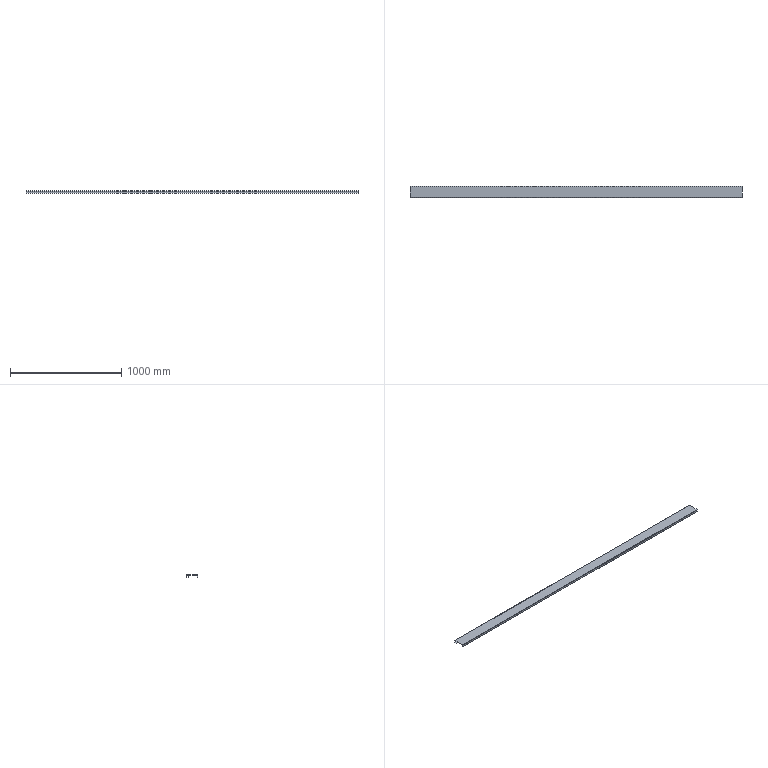Part | STEP file | E3-Transfer kettle guardrail 1 toe plate | 1 solid | 18 faces | box 2980 x 100 x 20 mm | volume 685013 mm3 | plane 12 | cylinder 6 | commonest cylinder face diameters 2 x3 5 x3
STEP:
#1=CARTESIAN_POINT('',(0.,0.,0.));
#2=DIRECTION('',(0.,0.,1.));
#3=DIRECTION('',(1.,0.,0.));
#4=AXIS2_PLACEMENT_3D('',#1,#2,#3);
#5=CARTESIAN_POINT('',(-1490.,1.5,-2.5));
#6=VERTEX_POINT('',#5);
#7=CARTESIAN_POINT('',(-1490.,1.5,-20.));
#8=VERTEX_POINT('',#7);
#9=CARTESIAN_POINT('',(-1490.,1.5,-2.5));
#10=DIRECTION('',(0.,0.,-1.));
#11=VECTOR('',#10,1.);
#12=LINE('',#9,#11);
#13=CARTESIAN_POINT('',(1490.,1.5,-2.5));
#14=DIRECTION('',(0.,-1.,0.));
#15=DIRECTION('',(0.,0.,1.));
#16=AXIS2_PLACEMENT_3D('',#13,#14,#15);
#17=PLANE('',#16);
#18=CARTESIAN_POINT('',(0.,2980.));
#19=DIRECTION('',(-1.,0.));
#20=VECTOR('',#19,1.);
#21=LINE('',#18,#20);
#22=(GEOMETRIC_REPRESENTATION_CONTEXT(2)PARAMETRIC_REPRESENTATION_CONTEXT()REPRESENTATION_CONTEXT('',''));
#23=DEFINITIONAL_REPRESENTATION('',(#21),#22);
#24=PCURVE('',#17,#23);
#25=CARTESIAN_POINT('',(-1490.,2.5,-2.5));
#26=DIRECTION('',(-1.,0.,0.));
#27=DIRECTION('',(0.,0.,-1.));
#28=AXIS2_PLACEMENT_3D('',#25,#26,#27);
#29=PLANE('',#28);
#30=CARTESIAN_POINT('',(0.,1.));
#31=DIRECTION('',(1.,0.));
#32=VECTOR('',#31,1.);
#33=LINE('',#30,#32);
#34=(GEOMETRIC_REPRESENTATION_CONTEXT(2)PARAMETRIC_REPRESENTATION_CONTEXT()REPRESENTATION_CONTEXT('',''));
#35=DEFINITIONAL_REPRESENTATION('',(#33),#34);
#36=PCURVE('',#29,#35);
#37=SURFACE_CURVE('',#12,(#24,#36),.PCURVE_S1.);
#38=EDGE_CURVE('',#6,#8,#37,.T.);
#39=ORIENTED_EDGE('',*,*,#38,.F.);
#40=CARTESIAN_POINT('',(1490.,1.5,-2.5));
#41=VERTEX_POINT('',#40);
#42=CARTESIAN_POINT('',(1490.,1.5,-2.5));
#43=DIRECTION('',(-1.,0.,0.));
#44=VECTOR('',#43,1.);
#45=LINE('',#42,#44);
#46=CARTESIAN_POINT('',(0.,0.));
#47=DIRECTION('',(0.,1.));
#48=VECTOR('',#47,1.);
#49=LINE('',#46,#48);
#50=(GEOMETRIC_REPRESENTATION_CONTEXT(2)PARAMETRIC_REPRESENTATION_CONTEXT()REPRESENTATION_CONTEXT('',''));
#51=DEFINITIONAL_REPRESENTATION('',(#49),#50);
#52=PCURVE('',#17,#51);
#53=CARTESIAN_POINT('',(1490.,2.5,-2.5));
#54=DIRECTION('',(-1.,0.,0.));
#55=DIRECTION('',(0.,0.,-1.));
#56=AXIS2_PLACEMENT_3D('',#53,#54,#55);
#57=CYLINDRICAL_SURFACE('',#56,1.);
#58=CARTESIAN_POINT('',(1.571,0.));
#59=DIRECTION('',(0.,1.));
#60=VECTOR('',#59,1.);
#61=LINE('',#58,#60);
#62=(GEOMETRIC_REPRESENTATION_CONTEXT(2)PARAMETRIC_REPRESENTATION_CONTEXT()REPRESENTATION_CONTEXT('',''));
#63=DEFINITIONAL_REPRESENTATION('',(#61),#62);
#64=PCURVE('',#57,#63);
#65=SURFACE_CURVE('',#45,(#52,#64),.PCURVE_S1.);
#66=EDGE_CURVE('',#41,#6,#65,.T.);
#67=ORIENTED_EDGE('',*,*,#66,.F.);
#68=CARTESIAN_POINT('',(1490.,1.5,-20.));
#69=VERTEX_POINT('',#68);
#70=CARTESIAN_POINT('',(1490.,1.5,-2.5));
#71=DIRECTION('',(0.,0.,-1.));
#72=VECTOR('',#71,1.);
#73=LINE('',#70,#72);
#74=CARTESIAN_POINT('',(0.,0.));
#75=DIRECTION('',(-1.,0.));
#76=VECTOR('',#75,1.);
#77=LINE('',#74,#76);
#78=(GEOMETRIC_REPRESENTATION_CONTEXT(2)PARAMETRIC_REPRESENTATION_CONTEXT()REPRESENTATION_CONTEXT('',''));
#79=DEFINITIONAL_REPRESENTATION('',(#77),#78);
#80=PCURVE('',#17,#79);
#81=CARTESIAN_POINT('',(1490.,2.5,-2.5));
#82=DIRECTION('',(-1.,0.,0.));
#83=DIRECTION('',(0.,0.,-1.));
#84=AXIS2_PLACEMENT_3D('',#81,#82,#83);
#85=PLANE('',#84);
#86=CARTESIAN_POINT('',(0.,1.));
#87=DIRECTION('',(1.,0.));
#88=VECTOR('',#87,1.);
#89=LINE('',#86,#88);
#90=(GEOMETRIC_REPRESENTATION_CONTEXT(2)PARAMETRIC_REPRESENTATION_CONTEXT()REPRESENTATION_CONTEXT('',''));
#91=DEFINITIONAL_REPRESENTATION('',(#89),#90);
#92=PCURVE('',#85,#91);
#93=SURFACE_CURVE('',#73,(#80,#92),.PCURVE_S1.);
#94=EDGE_CURVE('',#41,#69,#93,.T.);
#95=ORIENTED_EDGE('',*,*,#94,.T.);
#96=CARTESIAN_POINT('',(1490.,1.5,-20.));
#97=DIRECTION('',(-1.,0.,0.));
#98=VECTOR('',#97,1.);
#99=LINE('',#96,#98);
#100=CARTESIAN_POINT('',(-17.5,0.));
#101=DIRECTION('',(0.,1.));
#102=VECTOR('',#101,1.);
#103=LINE('',#100,#102);
#104=(GEOMETRIC_REPRESENTATION_CONTEXT(2)PARAMETRIC_REPRESENTATION_CONTEXT()REPRESENTATION_CONTEXT('',''));
#105=DEFINITIONAL_REPRESENTATION('',(#103),#104);
#106=PCURVE('',#17,#105);
#107=CARTESIAN_POINT('',(1490.,0.,-20.));
#108=DIRECTION('',(0.,0.,-1.));
#109=DIRECTION('',(1.,0.,0.));
#110=AXIS2_PLACEMENT_3D('',#107,#108,#109);
#111=PLANE('',#110);
#112=CARTESIAN_POINT('',(0.,-1.5));
#113=DIRECTION('',(-1.,0.));
#114=VECTOR('',#113,1.);
#115=LINE('',#112,#114);
#116=(GEOMETRIC_REPRESENTATION_CONTEXT(2)PARAMETRIC_REPRESENTATION_CONTEXT()REPRESENTATION_CONTEXT('',''));
#117=DEFINITIONAL_REPRESENTATION('',(#115),#116);
#118=PCURVE('',#111,#117);
#119=SURFACE_CURVE('',#99,(#106,#118),.PCURVE_S1.);
#120=EDGE_CURVE('',#69,#8,#119,.T.);
#121=ORIENTED_EDGE('',*,*,#120,.T.);
#122=EDGE_LOOP('',(#39,#67,#95,#121));
#123=FACE_BOUND('',#122,.T.);
#124=ADVANCED_FACE('',(#123),#17,.F.);
#125=CARTESIAN_POINT('',(-1490.,0.,-20.));
#126=VERTEX_POINT('',#125);
#127=CARTESIAN_POINT('',(-1490.,0.,-20.));
#128=DIRECTION('',(0.,1.,0.));
#129=VECTOR('',#128,1.);
#130=LINE('',#127,#129);
#131=CARTESIAN_POINT('',(-2980.,0.));
#132=DIRECTION('',(0.,-1.));
#133=VECTOR('',#132,1.);
#134=LINE('',#131,#133);
#135=(GEOMETRIC_REPRESENTATION_CONTEXT(2)PARAMETRIC_REPRESENTATION_CONTEXT()REPRESENTATION_CONTEXT('',''));
#136=DEFINITIONAL_REPRESENTATION('',(#134),#135);
#137=PCURVE('',#111,#136);
#138=CARTESIAN_POINT('',(17.5,2.5));
#139=DIRECTION('',(0.,-1.));
#140=VECTOR('',#139,1.);
#141=LINE('',#138,#140);
#142=(GEOMETRIC_REPRESENTATION_CONTEXT(2)PARAMETRIC_REPRESENTATION_CONTEXT()REPRESENTATION_CONTEXT('',''));
#143=DEFINITIONAL_REPRESENTATION('',(#141),#142);
#144=PCURVE('',#29,#143);
#145=SURFACE_CURVE('',#130,(#137,#144),.PCURVE_S1.);
#146=EDGE_CURVE('',#126,#8,#145,.T.);
#147=ORIENTED_EDGE('',*,*,#146,.T.);
#148=ORIENTED_EDGE('',*,*,#120,.F.);
#149=CARTESIAN_POINT('',(1490.,0.,-20.));
#150=VERTEX_POINT('',#149);
#151=CARTESIAN_POINT('',(1490.,0.,-20.));
#152=DIRECTION('',(0.,1.,0.));
#153=VECTOR('',#152,1.);
#154=LINE('',#151,#153);
#155=CARTESIAN_POINT('',(0.,0.));
#156=DIRECTION('',(0.,-1.));
#157=VECTOR('',#156,1.);
#158=LINE('',#155,#157);
#159=(GEOMETRIC_REPRESENTATION_CONTEXT(2)PARAMETRIC_REPRESENTATION_CONTEXT()REPRESENTATION_CONTEXT('',''));
#160=DEFINITIONAL_REPRESENTATION('',(#158),#159);
#161=PCURVE('',#111,#160);
#162=CARTESIAN_POINT('',(17.5,2.5));
#163=DIRECTION('',(0.,-1.));
#164=VECTOR('',#163,1.);
#165=LINE('',#162,#164);
#166=(GEOMETRIC_REPRESENTATION_CONTEXT(2)PARAMETRIC_REPRESENTATION_CONTEXT()REPRESENTATION_CONTEXT('',''));
#167=DEFINITIONAL_REPRESENTATION('',(#165),#166);
#168=PCURVE('',#85,#167);
#169=SURFACE_CURVE('',#154,(#161,#168),.PCURVE_S1.);
#170=EDGE_CURVE('',#150,#69,#169,.T.);
#171=ORIENTED_EDGE('',*,*,#170,.F.);
#172=CARTESIAN_POINT('',(1490.,0.,-20.));
#173=DIRECTION('',(-1.,0.,0.));
#174=VECTOR('',#173,1.);
#175=LINE('',#172,#174);
#176=CARTESIAN_POINT('',(0.,0.));
#177=DIRECTION('',(-1.,0.));
#178=VECTOR('',#177,1.);
#179=LINE('',#176,#178);
#180=(GEOMETRIC_REPRESENTATION_CONTEXT(2)PARAMETRIC_REPRESENTATION_CONTEXT()REPRESENTATION_CONTEXT('',''));
#181=DEFINITIONAL_REPRESENTATION('',(#179),#180);
#182=PCURVE('',#111,#181);
#183=CARTESIAN_POINT('',(1490.,0.,-2.5));
#184=DIRECTION('',(0.,-1.,0.));
#185=DIRECTION('',(0.,0.,1.));
#186=AXIS2_PLACEMENT_3D('',#183,#184,#185);
#187=PLANE('',#186);
#188=CARTESIAN_POINT('',(-17.5,0.));
#189=DIRECTION('',(0.,1.));
#190=VECTOR('',#189,1.);
#191=LINE('',#188,#190);
#192=(GEOMETRIC_REPRESENTATION_CONTEXT(2)PARAMETRIC_REPRESENTATION_CONTEXT()REPRESENTATION_CONTEXT('',''));
#193=DEFINITIONAL_REPRESENTATION('',(#191),#192);
#194=PCURVE('',#187,#193);
#195=SURFACE_CURVE('',#175,(#182,#194),.PCURVE_S1.);
#196=EDGE_CURVE('',#150,#126,#195,.T.);
#197=ORIENTED_EDGE('',*,*,#196,.T.);
#198=EDGE_LOOP('',(#147,#148,#171,#197));
#199=FACE_BOUND('',#198,.T.);
#200=ADVANCED_FACE('',(#199),#111,.T.);
#201=CARTESIAN_POINT('',(-1490.,0.,-2.5));
#202=VERTEX_POINT('',#201);
#203=CARTESIAN_POINT('',(-1490.,0.,-2.5));
#204=DIRECTION('',(0.,0.,-1.));
#205=VECTOR('',#204,1.);
#206=LINE('',#203,#205);
#207=CARTESIAN_POINT('',(0.,2980.));
#208=DIRECTION('',(-1.,0.));
#209=VECTOR('',#208,1.);
#210=LINE('',#207,#209);
#211=(GEOMETRIC_REPRESENTATION_CONTEXT(2)PARAMETRIC_REPRESENTATION_CONTEXT()REPRESENTATION_CONTEXT('',''));
#212=DEFINITIONAL_REPRESENTATION('',(#210),#211);
#213=PCURVE('',#187,#212);
#214=CARTESIAN_POINT('',(0.,2.5));
#215=DIRECTION('',(1.,0.));
#216=VECTOR('',#215,1.);
#217=LINE('',#214,#216);
#218=(GEOMETRIC_REPRESENTATION_CONTEXT(2)PARAMETRIC_REPRESENTATION_CONTEXT()REPRESENTATION_CONTEXT('',''));
#219=DEFINITIONAL_REPRESENTATION('',(#217),#218);
#220=PCURVE('',#29,#219);
#221=SURFACE_CURVE('',#206,(#213,#220),.PCURVE_S1.);
#222=EDGE_CURVE('',#202,#126,#221,.T.);
#223=ORIENTED_EDGE('',*,*,#222,.T.);
#224=ORIENTED_EDGE('',*,*,#196,.F.);
#225=CARTESIAN_POINT('',(1490.,0.,-2.5));
#226=VERTEX_POINT('',#225);
#227=CARTESIAN_POINT('',(1490.,0.,-2.5));
#228=DIRECTION('',(0.,0.,-1.));
#229=VECTOR('',#228,1.);
#230=LINE('',#227,#229);
#231=CARTESIAN_POINT('',(0.,0.));
#232=DIRECTION('',(-1.,0.));
#233=VECTOR('',#232,1.);
#234=LINE('',#231,#233);
#235=(GEOMETRIC_REPRESENTATION_CONTEXT(2)PARAMETRIC_REPRESENTATION_CONTEXT()REPRESENTATION_CONTEXT('',''));
#236=DEFINITIONAL_REPRESENTATION('',(#234),#235);
#237=PCURVE('',#187,#236);
#238=CARTESIAN_POINT('',(0.,2.5));
#239=DIRECTION('',(1.,0.));
#240=VECTOR('',#239,1.);
#241=LINE('',#238,#240);
#242=(GEOMETRIC_REPRESENTATION_CONTEXT(2)PARAMETRIC_REPRESENTATION_CONTEXT()REPRESENTATION_CONTEXT('',''));
#243=DEFINITIONAL_REPRESENTATION('',(#241),#242);
#244=PCURVE('',#85,#243);
#245=SURFACE_CURVE('',#230,(#237,#244),.PCURVE_S1.);
#246=EDGE_CURVE('',#226,#150,#245,.T.);
#247=ORIENTED_EDGE('',*,*,#246,.F.);
#248=CARTESIAN_POINT('',(1490.,0.,-2.5));
#249=DIRECTION('',(-1.,0.,0.));
#250=VECTOR('',#249,1.);
#251=LINE('',#248,#250);
#252=CARTESIAN_POINT('',(0.,0.));
#253=DIRECTION('',(0.,1.));
#254=VECTOR('',#253,1.);
#255=LINE('',#252,#254);
#256=(GEOMETRIC_REPRESENTATION_CONTEXT(2)PARAMETRIC_REPRESENTATION_CONTEXT()REPRESENTATION_CONTEXT('',''));
#257=DEFINITIONAL_REPRESENTATION('',(#255),#256);
#258=PCURVE('',#187,#257);
#259=CARTESIAN_POINT('',(1490.,2.5,-2.5));
#260=DIRECTION('',(-1.,0.,0.));
#261=DIRECTION('',(0.,0.,-1.));
#262=AXIS2_PLACEMENT_3D('',#259,#260,#261);
#263=CYLINDRICAL_SURFACE('',#262,2.5);
#264=CARTESIAN_POINT('',(1.571,0.));
#265=DIRECTION('',(0.,1.));
#266=VECTOR('',#265,1.);
#267=LINE('',#264,#266);
#268=(GEOMETRIC_REPRESENTATION_CONTEXT(2)PARAMETRIC_REPRESENTATION_CONTEXT()REPRESENTATION_CONTEXT('',''));
#269=DEFINITIONAL_REPRESENTATION('',(#267),#268);
#270=PCURVE('',#263,#269);
#271=SURFACE_CURVE('',#251,(#258,#270),.PCURVE_S1.);
#272=EDGE_CURVE('',#226,#202,#271,.T.);
#273=ORIENTED_EDGE('',*,*,#272,.T.);
#274=EDGE_LOOP('',(#223,#224,#247,#273));
#275=FACE_BOUND('',#274,.T.);
#276=ADVANCED_FACE('',(#275),#187,.T.);
#277=CARTESIAN_POINT('',(-1490.,2.5,0.));
#278=VERTEX_POINT('',#277);
#279=CARTESIAN_POINT('',(-1490.,2.5,-2.5));
#280=DIRECTION('',(1.,0.,0.));
#281=DIRECTION('',(0.,0.,-1.));
#282=AXIS2_PLACEMENT_3D('',#279,#280,#281);
#283=CIRCLE('',#282,2.5);
#284=CARTESIAN_POINT('',(6.283,2980.));
#285=DIRECTION('',(-1.,0.));
#286=VECTOR('',#285,1.);
#287=LINE('',#284,#286);
#288=(GEOMETRIC_REPRESENTATION_CONTEXT(2)PARAMETRIC_REPRESENTATION_CONTEXT()REPRESENTATION_CONTEXT('',''));
#289=DEFINITIONAL_REPRESENTATION('',(#287),#288);
#290=PCURVE('',#263,#289);
#291=CARTESIAN_POINT('',(2.5,0.));
#292=CARTESIAN_POINT('',(2.5,-4.33));
#293=CARTESIAN_POINT('',(-1.25,-2.165));
#294=CARTESIAN_POINT('',(-5.,0.));
#295=CARTESIAN_POINT('',(-1.25,2.165));
#296=CARTESIAN_POINT('',(2.5,4.33));
#297=CARTESIAN_POINT('',(2.5,0.));
#298=(BOUNDED_CURVE()B_SPLINE_CURVE(2,(#291,#292,#293,#294,#295,#296,#297),.UNSPECIFIED.,.T.,.F.)B_SPLINE_CURVE_WITH_KNOTS((1,2,2,2,2,1),(-2.094,0.,2.094,4.189,6.283,8.378),.UNSPECIFIED.)CURVE()GEOMETRIC_REPRESENTATION_ITEM()RATIONAL_B_SPLINE_CURVE((1.,0.5,1.,0.5,1.,0.5,1.))REPRESENTATION_ITEM(''));
#299=(GEOMETRIC_REPRESENTATION_CONTEXT(2)PARAMETRIC_REPRESENTATION_CONTEXT()REPRESENTATION_CONTEXT('',''));
#300=DEFINITIONAL_REPRESENTATION('',(#298),#299);
#301=PCURVE('',#29,#300);
#302=SURFACE_CURVE('',#283,(#290,#301),.PCURVE_S1.);
#303=EDGE_CURVE('',#278,#202,#302,.T.);
#304=ORIENTED_EDGE('',*,*,#303,.T.);
#305=ORIENTED_EDGE('',*,*,#272,.F.);
#306=CARTESIAN_POINT('',(1490.,2.5,0.));
#307=VERTEX_POINT('',#306);
#308=CARTESIAN_POINT('',(1490.,2.5,-2.5));
#309=DIRECTION('',(1.,0.,0.));
#310=DIRECTION('',(0.,0.,-1.));
#311=AXIS2_PLACEMENT_3D('',#308,#309,#310);
#312=CIRCLE('',#311,2.5);
#313=CARTESIAN_POINT('',(6.283,0.));
#314=DIRECTION('',(-1.,0.));
#315=VECTOR('',#314,1.);
#316=LINE('',#313,#315);
#317=(GEOMETRIC_REPRESENTATION_CONTEXT(2)PARAMETRIC_REPRESENTATION_CONTEXT()REPRESENTATION_CONTEXT('',''));
#318=DEFINITIONAL_REPRESENTATION('',(#316),#317);
#319=PCURVE('',#263,#318);
#320=CARTESIAN_POINT('',(2.5,0.));
#321=CARTESIAN_POINT('',(2.5,-4.33));
#322=CARTESIAN_POINT('',(-1.25,-2.165));
#323=CARTESIAN_POINT('',(-5.,0.));
#324=CARTESIAN_POINT('',(-1.25,2.165));
#325=CARTESIAN_POINT('',(2.5,4.33));
#326=CARTESIAN_POINT('',(2.5,0.));
#327=(BOUNDED_CURVE()B_SPLINE_CURVE(2,(#320,#321,#322,#323,#324,#325,#326),.UNSPECIFIED.,.T.,.F.)B_SPLINE_CURVE_WITH_KNOTS((1,2,2,2,2,1),(-2.094,0.,2.094,4.189,6.283,8.378),.UNSPECIFIED.)CURVE()GEOMETRIC_REPRESENTATION_ITEM()RATIONAL_B_SPLINE_CURVE((1.,0.5,1.,0.5,1.,0.5,1.))REPRESENTATION_ITEM(''));
#328=(GEOMETRIC_REPRESENTATION_CONTEXT(2)PARAMETRIC_REPRESENTATION_CONTEXT()REPRESENTATION_CONTEXT('',''));
#329=DEFINITIONAL_REPRESENTATION('',(#327),#328);
#330=PCURVE('',#85,#329);
#331=SURFACE_CURVE('',#312,(#319,#330),.PCURVE_S1.);
#332=EDGE_CURVE('',#307,#226,#331,.T.);
#333=ORIENTED_EDGE('',*,*,#332,.F.);
#334=CARTESIAN_POINT('',(1490.,2.5,0.));
#335=DIRECTION('',(-1.,0.,0.));
#336=VECTOR('',#335,1.);
#337=LINE('',#334,#336);
#338=CARTESIAN_POINT('',(3.142,0.));
#339=DIRECTION('',(0.,1.));
#340=VECTOR('',#339,1.);
#341=LINE('',#338,#340);
#342=(GEOMETRIC_REPRESENTATION_CONTEXT(2)PARAMETRIC_REPRESENTATION_CONTEXT()REPRESENTATION_CONTEXT('',''));
#343=DEFINITIONAL_REPRESENTATION('',(#341),#342);
#344=PCURVE('',#263,#343);
#345=CARTESIAN_POINT('',(1490.,2.5,0.));
#346=DIRECTION('',(0.,0.,1.));
#347=DIRECTION('',(-1.,0.,0.));
#348=AXIS2_PLACEMENT_3D('',#345,#346,#347);
#349=PLANE('',#348);
#350=CARTESIAN_POINT('',(0.,0.));
#351=DIRECTION('',(1.,0.));
#352=VECTOR('',#351,1.);
#353=LINE('',#350,#352);
#354=(GEOMETRIC_REPRESENTATION_CONTEXT(2)PARAMETRIC_REPRESENTATION_CONTEXT()REPRESENTATION_CONTEXT('',''));
#355=DEFINITIONAL_REPRESENTATION('',(#353),#354);
#356=PCURVE('',#349,#355);
#357=SURFACE_CURVE('',#337,(#344,#356),.PCURVE_S1.);
#358=EDGE_CURVE('',#307,#278,#357,.T.);
#359=ORIENTED_EDGE('',*,*,#358,.T.);
#360=EDGE_LOOP('',(#304,#305,#333,#359));
#361=FACE_BOUND('',#360,.T.);
#362=ADVANCED_FACE('',(#361),#263,.T.);
#363=CARTESIAN_POINT('',(-1490.,97.5,0.));
#364=VERTEX_POINT('',#363);
#365=CARTESIAN_POINT('',(-1490.,2.5,0.));
#366=DIRECTION('',(0.,-1.,0.));
#367=VECTOR('',#366,1.);
#368=LINE('',#365,#367);
#369=CARTESIAN_POINT('',(2980.,0.));
#370=DIRECTION('',(0.,1.));
#371=VECTOR('',#370,1.);
#372=LINE('',#369,#371);
#373=(GEOMETRIC_REPRESENTATION_CONTEXT(2)PARAMETRIC_REPRESENTATION_CONTEXT()REPRESENTATION_CONTEXT('',''));
#374=DEFINITIONAL_REPRESENTATION('',(#372),#373);
#375=PCURVE('',#349,#374);
#376=CARTESIAN_POINT('',(-2.5,0.));
#377=DIRECTION('',(0.,1.));
#378=VECTOR('',#377,1.);
#379=LINE('',#376,#378);
#380=(GEOMETRIC_REPRESENTATION_CONTEXT(2)PARAMETRIC_REPRESENTATION_CONTEXT()REPRESENTATION_CONTEXT('',''));
#381=DEFINITIONAL_REPRESENTATION('',(#379),#380);
#382=PCURVE('',#29,#381);
#383=SURFACE_CURVE('',#368,(#375,#382),.PCURVE_S1.);
#384=EDGE_CURVE('',#364,#278,#383,.T.);
#385=ORIENTED_EDGE('',*,*,#384,.T.);
#386=ORIENTED_EDGE('',*,*,#358,.F.);
#387=CARTESIAN_POINT('',(1490.,97.5,0.));
#388=VERTEX_POINT('',#387);
#389=CARTESIAN_POINT('',(1490.,2.5,0.));
#390=DIRECTION('',(0.,-1.,0.));
#391=VECTOR('',#390,1.);
#392=LINE('',#389,#391);
#393=CARTESIAN_POINT('',(0.,0.));
#394=DIRECTION('',(0.,1.));
#395=VECTOR('',#394,1.);
#396=LINE('',#393,#395);
#397=(GEOMETRIC_REPRESENTATION_CONTEXT(2)PARAMETRIC_REPRESENTATION_CONTEXT()REPRESENTATION_CONTEXT('',''));
#398=DEFINITIONAL_REPRESENTATION('',(#396),#397);
#399=PCURVE('',#349,#398);
#400=CARTESIAN_POINT('',(-2.5,0.));
#401=DIRECTION('',(0.,1.));
#402=VECTOR('',#401,1.);
#403=LINE('',#400,#402);
#404=(GEOMETRIC_REPRESENTATION_CONTEXT(2)PARAMETRIC_REPRESENTATION_CONTEXT()REPRESENTATION_CONTEXT('',''));
#405=DEFINITIONAL_REPRESENTATION('',(#403),#404);
#406=PCURVE('',#85,#405);
#407=SURFACE_CURVE('',#392,(#399,#406),.PCURVE_S1.);
#408=EDGE_CURVE('',#388,#307,#407,.T.);
#409=ORIENTED_EDGE('',*,*,#408,.F.);
#410=CARTESIAN_POINT('',(1490.,97.5,0.));
#411=DIRECTION('',(-1.,0.,0.));
#412=VECTOR('',#411,1.);
#413=LINE('',#410,#412);
#414=CARTESIAN_POINT('',(0.,-95.));
#415=DIRECTION('',(1.,0.));
#416=VECTOR('',#415,1.);
#417=LINE('',#414,#416);
#418=(GEOMETRIC_REPRESENTATION_CONTEXT(2)PARAMETRIC_REPRESENTATION_CONTEXT()REPRESENTATION_CONTEXT('',''));
#419=DEFINITIONAL_REPRESENTATION('',(#417),#418);
#420=PCURVE('',#349,#419);
#421=CARTESIAN_POINT('',(1490.,97.5,-2.5));
#422=DIRECTION('',(-1.,0.,0.));
#423=DIRECTION('',(0.,0.,-1.));
#424=AXIS2_PLACEMENT_3D('',#421,#422,#423);
#425=CYLINDRICAL_SURFACE('',#424,2.5);
#426=CARTESIAN_POINT('',(3.142,0.));
#427=DIRECTION('',(0.,1.));
#428=VECTOR('',#427,1.);
#429=LINE('',#426,#428);
#430=(GEOMETRIC_REPRESENTATION_CONTEXT(2)PARAMETRIC_REPRESENTATION_CONTEXT()REPRESENTATION_CONTEXT('',''));
#431=DEFINITIONAL_REPRESENTATION('',(#429),#430);
#432=PCURVE('',#425,#431);
#433=SURFACE_CURVE('',#413,(#420,#432),.PCURVE_S1.);
#434=EDGE_CURVE('',#388,#364,#433,.T.);
#435=ORIENTED_EDGE('',*,*,#434,.T.);
#436=EDGE_LOOP('',(#385,#386,#409,#435));
#437=FACE_BOUND('',#436,.T.);
#438=ADVANCED_FACE('',(#437),#349,.T.);
#439=CARTESIAN_POINT('',(-1490.,100.,-2.5));
#440=VERTEX_POINT('',#439);
#441=CARTESIAN_POINT('',(-1490.,97.5,-2.5));
#442=DIRECTION('',(1.,0.,0.));
#443=DIRECTION('',(0.,0.,1.));
#444=AXIS2_PLACEMENT_3D('',#441,#442,#443);
#445=CIRCLE('',#444,2.5);
#446=CARTESIAN_POINT('',(9.425,2980.));
#447=DIRECTION('',(-1.,0.));
#448=VECTOR('',#447,1.);
#449=LINE('',#446,#448);
#450=(GEOMETRIC_REPRESENTATION_CONTEXT(2)PARAMETRIC_REPRESENTATION_CONTEXT()REPRESENTATION_CONTEXT('',''));
#451=DEFINITIONAL_REPRESENTATION('',(#449),#450);
#452=PCURVE('',#425,#451);
#453=CARTESIAN_POINT('',(-2.5,-95.));
#454=CARTESIAN_POINT('',(-2.5,-90.67));
#455=CARTESIAN_POINT('',(1.25,-92.835));
#456=CARTESIAN_POINT('',(5.,-95.));
#457=CARTESIAN_POINT('',(1.25,-97.165));
#458=CARTESIAN_POINT('',(-2.5,-99.33));
#459=CARTESIAN_POINT('',(-2.5,-95.));
#460=(BOUNDED_CURVE()B_SPLINE_CURVE(2,(#453,#454,#455,#456,#457,#458,#459),.UNSPECIFIED.,.T.,.F.)B_SPLINE_CURVE_WITH_KNOTS((1,2,2,2,2,1),(-2.094,0.,2.094,4.189,6.283,8.378),.UNSPECIFIED.)CURVE()GEOMETRIC_REPRESENTATION_ITEM()RATIONAL_B_SPLINE_CURVE((1.,0.5,1.,0.5,1.,0.5,1.))REPRESENTATION_ITEM(''));
#461=(GEOMETRIC_REPRESENTATION_CONTEXT(2)PARAMETRIC_REPRESENTATION_CONTEXT()REPRESENTATION_CONTEXT('',''));
#462=DEFINITIONAL_REPRESENTATION('',(#460),#461);
#463=PCURVE('',#29,#462);
#464=SURFACE_CURVE('',#445,(#452,#463),.PCURVE_S1.);
#465=EDGE_CURVE('',#440,#364,#464,.T.);
#466=ORIENTED_EDGE('',*,*,#465,.T.);
#467=ORIENTED_EDGE('',*,*,#434,.F.);
#468=CARTESIAN_POINT('',(1490.,100.,-2.5));
#469=VERTEX_POINT('',#468);
#470=CARTESIAN_POINT('',(1490.,97.5,-2.5));
#471=DIRECTION('',(1.,0.,0.));
#472=DIRECTION('',(0.,0.,1.));
#473=AXIS2_PLACEMENT_3D('',#470,#471,#472);
#474=CIRCLE('',#473,2.5);
#475=CARTESIAN_POINT('',(9.425,0.));
#476=DIRECTION('',(-1.,0.));
#477=VECTOR('',#476,1.);
#478=LINE('',#475,#477);
#479=(GEOMETRIC_REPRESENTATION_CONTEXT(2)PARAMETRIC_REPRESENTATION_CONTEXT()REPRESENTATION_CONTEXT('',''));
#480=DEFINITIONAL_REPRESENTATION('',(#478),#479);
#481=PCURVE('',#425,#480);
#482=CARTESIAN_POINT('',(-2.5,-95.));
#483=CARTESIAN_POINT('',(-2.5,-90.67));
#484=CARTESIAN_POINT('',(1.25,-92.835));
#485=CARTESIAN_POINT('',(5.,-95.));
#486=CARTESIAN_POINT('',(1.25,-97.165));
#487=CARTESIAN_POINT('',(-2.5,-99.33));
#488=CARTESIAN_POINT('',(-2.5,-95.));
#489=(BOUNDED_CURVE()B_SPLINE_CURVE(2,(#482,#483,#484,#485,#486,#487,#488),.UNSPECIFIED.,.T.,.F.)B_SPLINE_CURVE_WITH_KNOTS((1,2,2,2,2,1),(-2.094,0.,2.094,4.189,6.283,8.378),.UNSPECIFIED.)CURVE()GEOMETRIC_REPRESENTATION_ITEM()RATIONAL_B_SPLINE_CURVE((1.,0.5,1.,0.5,1.,0.5,1.))REPRESENTATION_ITEM(''));
#490=(GEOMETRIC_REPRESENTATION_CONTEXT(2)PARAMETRIC_REPRESENTATION_CONTEXT()REPRESENTATION_CONTEXT('',''));
#491=DEFINITIONAL_REPRESENTATION('',(#489),#490);
#492=PCURVE('',#85,#491);
#493=SURFACE_CURVE('',#474,(#481,#492),.PCURVE_S1.);
#494=EDGE_CURVE('',#469,#388,#493,.T.);
#495=ORIENTED_EDGE('',*,*,#494,.F.);
#496=CARTESIAN_POINT('',(1490.,100.,-2.5));
#497=DIRECTION('',(-1.,0.,0.));
#498=VECTOR('',#497,1.);
#499=LINE('',#496,#498);
#500=CARTESIAN_POINT('',(4.712,0.));
#501=DIRECTION('',(0.,1.));
#502=VECTOR('',#501,1.);
#503=LINE('',#500,#502);
#504=(GEOMETRIC_REPRESENTATION_CONTEXT(2)PARAMETRIC_REPRESENTATION_CONTEXT()REPRESENTATION_CONTEXT('',''));
#505=DEFINITIONAL_REPRESENTATION('',(#503),#504);
#506=PCURVE('',#425,#505);
#507=CARTESIAN_POINT('',(1490.,100.,-2.5));
#508=DIRECTION('',(0.,1.,0.));
#509=DIRECTION('',(0.,0.,-1.));
#510=AXIS2_PLACEMENT_3D('',#507,#508,#509);
#511=PLANE('',#510);
#512=CARTESIAN_POINT('',(0.,0.));
#513=DIRECTION('',(0.,1.));
#514=VECTOR('',#513,1.);
#515=LINE('',#512,#514);
#516=(GEOMETRIC_REPRESENTATION_CONTEXT(2)PARAMETRIC_REPRESENTATION_CONTEXT()REPRESENTATION_CONTEXT('',''));
#517=DEFINITIONAL_REPRESENTATION('',(#515),#516);
#518=PCURVE('',#511,#517);
#519=SURFACE_CURVE('',#499,(#506,#518),.PCURVE_S1.);
#520=EDGE_CURVE('',#469,#440,#519,.T.);
#521=ORIENTED_EDGE('',*,*,#520,.T.);
#522=EDGE_LOOP('',(#466,#467,#495,#521));
#523=FACE_BOUND('',#522,.T.);
#524=ADVANCED_FACE('',(#523),#425,.T.);
#525=CARTESIAN_POINT('',(-1490.,100.,-17.5));
#526=VERTEX_POINT('',#525);
#527=CARTESIAN_POINT('',(-1490.,100.,-2.5));
#528=DIRECTION('',(0.,0.,1.));
#529=VECTOR('',#528,1.);
#530=LINE('',#527,#529);
#531=CARTESIAN_POINT('',(0.,2980.));
#532=DIRECTION('',(-1.,0.));
#533=VECTOR('',#532,1.);
#534=LINE('',#531,#533);
#535=(GEOMETRIC_REPRESENTATION_CONTEXT(2)PARAMETRIC_REPRESENTATION_CONTEXT()REPRESENTATION_CONTEXT('',''));
#536=DEFINITIONAL_REPRESENTATION('',(#534),#535);
#537=PCURVE('',#511,#536);
#538=CARTESIAN_POINT('',(0.,-97.5));
#539=DIRECTION('',(-1.,0.));
#540=VECTOR('',#539,1.);
#541=LINE('',#538,#540);
#542=(GEOMETRIC_REPRESENTATION_CONTEXT(2)PARAMETRIC_REPRESENTATION_CONTEXT()REPRESENTATION_CONTEXT('',''));
#543=DEFINITIONAL_REPRESENTATION('',(#541),#542);
#544=PCURVE('',#29,#543);
#545=SURFACE_CURVE('',#530,(#537,#544),.PCURVE_S1.);
#546=EDGE_CURVE('',#526,#440,#545,.T.);
#547=ORIENTED_EDGE('',*,*,#546,.T.);
#548=ORIENTED_EDGE('',*,*,#520,.F.);
#549=CARTESIAN_POINT('',(1490.,100.,-17.5));
#550=VERTEX_POINT('',#549);
#551=CARTESIAN_POINT('',(1490.,100.,-2.5));
#552=DIRECTION('',(0.,0.,1.));
#553=VECTOR('',#552,1.);
#554=LINE('',#551,#553);
#555=CARTESIAN_POINT('',(0.,0.));
#556=DIRECTION('',(-1.,0.));
#557=VECTOR('',#556,1.);
#558=LINE('',#555,#557);
#559=(GEOMETRIC_REPRESENTATION_CONTEXT(2)PARAMETRIC_REPRESENTATION_CONTEXT()REPRESENTATION_CONTEXT('',''));
#560=DEFINITIONAL_REPRESENTATION('',(#558),#559);
#561=PCURVE('',#511,#560);
#562=CARTESIAN_POINT('',(0.,-97.5));
#563=DIRECTION('',(-1.,0.));
#564=VECTOR('',#563,1.);
#565=LINE('',#562,#564);
#566=(GEOMETRIC_REPRESENTATION_CONTEXT(2)PARAMETRIC_REPRESENTATION_CONTEXT()REPRESENTATION_CONTEXT('',''));
#567=DEFINITIONAL_REPRESENTATION('',(#565),#566);
#568=PCURVE('',#85,#567);
#569=SURFACE_CURVE('',#554,(#561,#568),.PCURVE_S1.);
#570=EDGE_CURVE('',#550,#469,#569,.T.);
#571=ORIENTED_EDGE('',*,*,#570,.F.);
#572=CARTESIAN_POINT('',(1490.,100.,-17.5));
#573=DIRECTION('',(-1.,0.,0.));
#574=VECTOR('',#573,1.);
#575=LINE('',#572,#574);
#576=CARTESIAN_POINT('',(15.,0.));
#577=DIRECTION('',(0.,1.));
#578=VECTOR('',#577,1.);
#579=LINE('',#576,#578);
#580=(GEOMETRIC_REPRESENTATION_CONTEXT(2)PARAMETRIC_REPRESENTATION_CONTEXT()REPRESENTATION_CONTEXT('',''));
#581=DEFINITIONAL_REPRESENTATION('',(#579),#580);
#582=PCURVE('',#511,#581);
#583=CARTESIAN_POINT('',(1490.,97.5,-17.5));
#584=DIRECTION('',(-1.,0.,0.));
#585=DIRECTION('',(0.,0.,-1.));
#586=AXIS2_PLACEMENT_3D('',#583,#584,#585);
#587=CYLINDRICAL_SURFACE('',#586,2.5);
#588=CARTESIAN_POINT('',(4.712,0.));
#589=DIRECTION('',(0.,1.));
#590=VECTOR('',#589,1.);
#591=LINE('',#588,#590);
#592=(GEOMETRIC_REPRESENTATION_CONTEXT(2)PARAMETRIC_REPRESENTATION_CONTEXT()REPRESENTATION_CONTEXT('',''));
#593=DEFINITIONAL_REPRESENTATION('',(#591),#592);
#594=PCURVE('',#587,#593);
#595=SURFACE_CURVE('',#575,(#582,#594),.PCURVE_S1.);
#596=EDGE_CURVE('',#550,#526,#595,.T.);
#597=ORIENTED_EDGE('',*,*,#596,.T.);
#598=EDGE_LOOP('',(#547,#548,#571,#597));
#599=FACE_BOUND('',#598,.T.);
#600=ADVANCED_FACE('',(#599),#511,.T.);
#601=CARTESIAN_POINT('',(-1490.,97.5,-20.));
#602=VERTEX_POINT('',#601);
#603=CARTESIAN_POINT('',(-1490.,97.5,-17.5));
#604=DIRECTION('',(1.,0.,0.));
#605=DIRECTION('',(0.,0.,1.));
#606=AXIS2_PLACEMENT_3D('',#603,#604,#605);
#607=CIRCLE('',#606,2.5);
#608=CARTESIAN_POINT('',(9.425,2980.));
#609=DIRECTION('',(-1.,0.));
#610=VECTOR('',#609,1.);
#611=LINE('',#608,#610);
#612=(GEOMETRIC_REPRESENTATION_CONTEXT(2)PARAMETRIC_REPRESENTATION_CONTEXT()REPRESENTATION_CONTEXT('',''));
#613=DEFINITIONAL_REPRESENTATION('',(#611),#612);
#614=PCURVE('',#587,#613);
#615=CARTESIAN_POINT('',(12.5,-95.));
#616=CARTESIAN_POINT('',(12.5,-90.67));
#617=CARTESIAN_POINT('',(16.25,-92.835));
#618=CARTESIAN_POINT('',(20.,-95.));
#619=CARTESIAN_POINT('',(16.25,-97.165));
#620=CARTESIAN_POINT('',(12.5,-99.33));
#621=CARTESIAN_POINT('',(12.5,-95.));
#622=(BOUNDED_CURVE()B_SPLINE_CURVE(2,(#615,#616,#617,#618,#619,#620,#621),.UNSPECIFIED.,.T.,.F.)B_SPLINE_CURVE_WITH_KNOTS((1,2,2,2,2,1),(-2.094,0.,2.094,4.189,6.283,8.378),.UNSPECIFIED.)CURVE()GEOMETRIC_REPRESENTATION_ITEM()RATIONAL_B_SPLINE_CURVE((1.,0.5,1.,0.5,1.,0.5,1.))REPRESENTATION_ITEM(''));
#623=(GEOMETRIC_REPRESENTATION_CONTEXT(2)PARAMETRIC_REPRESENTATION_CONTEXT()REPRESENTATION_CONTEXT('',''));
#624=DEFINITIONAL_REPRESENTATION('',(#622),#623);
#625=PCURVE('',#29,#624);
#626=SURFACE_CURVE('',#607,(#614,#625),.PCURVE_S1.);
#627=EDGE_CURVE('',#602,#526,#626,.T.);
#628=ORIENTED_EDGE('',*,*,#627,.T.);
#629=ORIENTED_EDGE('',*,*,#596,.F.);
#630=CARTESIAN_POINT('',(1490.,97.5,-20.));
#631=VERTEX_POINT('',#630);
#632=CARTESIAN_POINT('',(1490.,97.5,-17.5));
#633=DIRECTION('',(1.,0.,0.));
#634=DIRECTION('',(0.,0.,1.));
#635=AXIS2_PLACEMENT_3D('',#632,#633,#634);
#636=CIRCLE('',#635,2.5);
#637=CARTESIAN_POINT('',(9.425,0.));
#638=DIRECTION('',(-1.,0.));
#639=VECTOR('',#638,1.);
#640=LINE('',#637,#639);
#641=(GEOMETRIC_REPRESENTATION_CONTEXT(2)PARAMETRIC_REPRESENTATION_CONTEXT()REPRESENTATION_CONTEXT('',''));
#642=DEFINITIONAL_REPRESENTATION('',(#640),#641);
#643=PCURVE('',#587,#642);
#644=CARTESIAN_POINT('',(12.5,-95.));
#645=CARTESIAN_POINT('',(12.5,-90.67));
#646=CARTESIAN_POINT('',(16.25,-92.835));
#647=CARTESIAN_POINT('',(20.,-95.));
#648=CARTESIAN_POINT('',(16.25,-97.165));
#649=CARTESIAN_POINT('',(12.5,-99.33));
#650=CARTESIAN_POINT('',(12.5,-95.));
#651=(BOUNDED_CURVE()B_SPLINE_CURVE(2,(#644,#645,#646,#647,#648,#649,#650),.UNSPECIFIED.,.T.,.F.)B_SPLINE_CURVE_WITH_KNOTS((1,2,2,2,2,1),(-2.094,0.,2.094,4.189,6.283,8.378),.UNSPECIFIED.)CURVE()GEOMETRIC_REPRESENTATION_ITEM()RATIONAL_B_SPLINE_CURVE((1.,0.5,1.,0.5,1.,0.5,1.))REPRESENTATION_ITEM(''));
#652=(GEOMETRIC_REPRESENTATION_CONTEXT(2)PARAMETRIC_REPRESENTATION_CONTEXT()REPRESENTATION_CONTEXT('',''));
#653=DEFINITIONAL_REPRESENTATION('',(#651),#652);
#654=PCURVE('',#85,#653);
#655=SURFACE_CURVE('',#636,(#643,#654),.PCURVE_S1.);
#656=EDGE_CURVE('',#631,#550,#655,.T.);
#657=ORIENTED_EDGE('',*,*,#656,.F.);
#658=CARTESIAN_POINT('',(1490.,97.5,-20.));
#659=DIRECTION('',(-1.,0.,0.));
#660=VECTOR('',#659,1.);
#661=LINE('',#658,#660);
#662=CARTESIAN_POINT('',(6.283,0.));
#663=DIRECTION('',(0.,1.));
#664=VECTOR('',#663,1.);
#665=LINE('',#662,#664);
#666=(GEOMETRIC_REPRESENTATION_CONTEXT(2)PARAMETRIC_REPRESENTATION_CONTEXT()REPRESENTATION_CONTEXT('',''));
#667=DEFINITIONAL_REPRESENTATION('',(#665),#666);
#668=PCURVE('',#587,#667);
#669=CARTESIAN_POINT('',(1490.,97.5,-20.));
#670=DIRECTION('',(0.,0.,-1.));
#671=DIRECTION('',(1.,0.,0.));
#672=AXIS2_PLACEMENT_3D('',#669,#670,#671);
#673=PLANE('',#672);
#674=CARTESIAN_POINT('',(0.,0.));
#675=DIRECTION('',(-1.,0.));
#676=VECTOR('',#675,1.);
#677=LINE('',#674,#676);
#678=(GEOMETRIC_REPRESENTATION_CONTEXT(2)PARAMETRIC_REPRESENTATION_CONTEXT()REPRESENTATION_CONTEXT('',''));
#679=DEFINITIONAL_REPRESENTATION('',(#677),#678);
#680=PCURVE('',#673,#679);
#681=SURFACE_CURVE('',#661,(#668,#680),.PCURVE_S1.);
#682=EDGE_CURVE('',#631,#602,#681,.T.);
#683=ORIENTED_EDGE('',*,*,#682,.T.);
#684=EDGE_LOOP('',(#628,#629,#657,#683));
#685=FACE_BOUND('',#684,.T.);
#686=ADVANCED_FACE('',(#685),#587,.T.);
#687=CARTESIAN_POINT('',(-1490.,80.,-20.));
#688=VERTEX_POINT('',#687);
#689=CARTESIAN_POINT('',(-1490.,97.5,-20.));
#690=DIRECTION('',(0.,1.,0.));
#691=VECTOR('',#690,1.);
#692=LINE('',#689,#691);
#693=CARTESIAN_POINT('',(-2980.,0.));
#694=DIRECTION('',(0.,-1.));
#695=VECTOR('',#694,1.);
#696=LINE('',#693,#695);
#697=(GEOMETRIC_REPRESENTATION_CONTEXT(2)PARAMETRIC_REPRESENTATION_CONTEXT()REPRESENTATION_CONTEXT('',''));
#698=DEFINITIONAL_REPRESENTATION('',(#696),#697);
#699=PCURVE('',#673,#698);
#700=CARTESIAN_POINT('',(17.5,-95.));
#701=DIRECTION('',(0.,-1.));
#702=VECTOR('',#701,1.);
#703=LINE('',#700,#702);
#704=(GEOMETRIC_REPRESENTATION_CONTEXT(2)PARAMETRIC_REPRESENTATION_CONTEXT()REPRESENTATION_CONTEXT('',''));
#705=DEFINITIONAL_REPRESENTATION('',(#703),#704);
#706=PCURVE('',#29,#705);
#707=SURFACE_CURVE('',#692,(#699,#706),.PCURVE_S1.);
#708=EDGE_CURVE('',#688,#602,#707,.T.);
#709=ORIENTED_EDGE('',*,*,#708,.T.);
#710=ORIENTED_EDGE('',*,*,#682,.F.);
#711=CARTESIAN_POINT('',(1490.,80.,-20.));
#712=VERTEX_POINT('',#711);
#713=CARTESIAN_POINT('',(1490.,97.5,-20.));
#714=DIRECTION('',(0.,1.,0.));
#715=VECTOR('',#714,1.);
#716=LINE('',#713,#715);
#717=CARTESIAN_POINT('',(0.,0.));
#718=DIRECTION('',(0.,-1.));
#719=VECTOR('',#718,1.);
#720=LINE('',#717,#719);
#721=(GEOMETRIC_REPRESENTATION_CONTEXT(2)PARAMETRIC_REPRESENTATION_CONTEXT()REPRESENTATION_CONTEXT('',''));
#722=DEFINITIONAL_REPRESENTATION('',(#720),#721);
#723=PCURVE('',#673,#722);
#724=CARTESIAN_POINT('',(17.5,-95.));
#725=DIRECTION('',(0.,-1.));
#726=VECTOR('',#725,1.);
#727=LINE('',#724,#726);
#728=(GEOMETRIC_REPRESENTATION_CONTEXT(2)PARAMETRIC_REPRESENTATION_CONTEXT()REPRESENTATION_CONTEXT('',''));
#729=DEFINITIONAL_REPRESENTATION('',(#727),#728);
#730=PCURVE('',#85,#729);
#731=SURFACE_CURVE('',#716,(#723,#730),.PCURVE_S1.);
#732=EDGE_CURVE('',#712,#631,#731,.T.);
#733=ORIENTED_EDGE('',*,*,#732,.F.);
#734=CARTESIAN_POINT('',(1490.,80.,-20.));
#735=DIRECTION('',(-1.,0.,0.));
#736=VECTOR('',#735,1.);
#737=LINE('',#734,#736);
#738=CARTESIAN_POINT('',(0.,17.5));
#739=DIRECTION('',(-1.,0.));
#740=VECTOR('',#739,1.);
#741=LINE('',#738,#740);
#742=(GEOMETRIC_REPRESENTATION_CONTEXT(2)PARAMETRIC_REPRESENTATION_CONTEXT()REPRESENTATION_CONTEXT('',''));
#743=DEFINITIONAL_REPRESENTATION('',(#741),#742);
#744=PCURVE('',#673,#743);
#745=CARTESIAN_POINT('',(1490.,80.,-18.5));
#746=DIRECTION('',(0.,-1.,0.));
#747=DIRECTION('',(0.,0.,1.));
#748=AXIS2_PLACEMENT_3D('',#745,#746,#747);
#749=PLANE('',#748);
#750=CARTESIAN_POINT('',(-1.5,0.));
#751=DIRECTION('',(0.,1.));
#752=VECTOR('',#751,1.);
#753=LINE('',#750,#752);
#754=(GEOMETRIC_REPRESENTATION_CONTEXT(2)PARAMETRIC_REPRESENTATION_CONTEXT()REPRESENTATION_CONTEXT('',''));
#755=DEFINITIONAL_REPRESENTATION('',(#753),#754);
#756=PCURVE('',#749,#755);
#757=SURFACE_CURVE('',#737,(#744,#756),.PCURVE_S1.);
#758=EDGE_CURVE('',#712,#688,#757,.T.);
#759=ORIENTED_EDGE('',*,*,#758,.T.);
#760=EDGE_LOOP('',(#709,#710,#733,#759));
#761=FACE_BOUND('',#760,.T.);
#762=ADVANCED_FACE('',(#761),#673,.T.);
#763=CARTESIAN_POINT('',(-1490.,80.,-18.5));
#764=VERTEX_POINT('',#763);
#765=CARTESIAN_POINT('',(-1490.,80.,-18.5));
#766=DIRECTION('',(0.,0.,-1.));
#767=VECTOR('',#766,1.);
#768=LINE('',#765,#767);
#769=CARTESIAN_POINT('',(0.,2980.));
#770=DIRECTION('',(-1.,0.));
#771=VECTOR('',#770,1.);
#772=LINE('',#769,#771);
#773=(GEOMETRIC_REPRESENTATION_CONTEXT(2)PARAMETRIC_REPRESENTATION_CONTEXT()REPRESENTATION_CONTEXT('',''));
#774=DEFINITIONAL_REPRESENTATION('',(#772),#773);
#775=PCURVE('',#749,#774);
#776=CARTESIAN_POINT('',(16.,-77.5));
#777=DIRECTION('',(1.,0.));
#778=VECTOR('',#777,1.);
#779=LINE('',#776,#778);
#780=(GEOMETRIC_REPRESENTATION_CONTEXT(2)PARAMETRIC_REPRESENTATION_CONTEXT()REPRESENTATION_CONTEXT('',''));
#781=DEFINITIONAL_REPRESENTATION('',(#779),#780);
#782=PCURVE('',#29,#781);
#783=SURFACE_CURVE('',#768,(#775,#782),.PCURVE_S1.);
#784=EDGE_CURVE('',#764,#688,#783,.T.);
#785=ORIENTED_EDGE('',*,*,#784,.T.);
#786=ORIENTED_EDGE('',*,*,#758,.F.);
#787=CARTESIAN_POINT('',(1490.,80.,-18.5));
#788=VERTEX_POINT('',#787);
#789=CARTESIAN_POINT('',(1490.,80.,-18.5));
#790=DIRECTION('',(0.,0.,-1.));
#791=VECTOR('',#790,1.);
#792=LINE('',#789,#791);
#793=CARTESIAN_POINT('',(0.,0.));
#794=DIRECTION('',(-1.,0.));
#795=VECTOR('',#794,1.);
#796=LINE('',#793,#795);
#797=(GEOMETRIC_REPRESENTATION_CONTEXT(2)PARAMETRIC_REPRESENTATION_CONTEXT()REPRESENTATION_CONTEXT('',''));
#798=DEFINITIONAL_REPRESENTATION('',(#796),#797);
#799=PCURVE('',#749,#798);
#800=CARTESIAN_POINT('',(16.,-77.5));
#801=DIRECTION('',(1.,0.));
#802=VECTOR('',#801,1.);
#803=LINE('',#800,#802);
#804=(GEOMETRIC_REPRESENTATION_CONTEXT(2)PARAMETRIC_REPRESENTATION_CONTEXT()REPRESENTATION_CONTEXT('',''));
#805=DEFINITIONAL_REPRESENTATION('',(#803),#804);
#806=PCURVE('',#85,#805);
#807=SURFACE_CURVE('',#792,(#799,#806),.PCURVE_S1.);
#808=EDGE_CURVE('',#788,#712,#807,.T.);
#809=ORIENTED_EDGE('',*,*,#808,.F.);
#810=CARTESIAN_POINT('',(1490.,80.,-18.5));
#811=DIRECTION('',(-1.,0.,0.));
#812=VECTOR('',#811,1.);
#813=LINE('',#810,#812);
#814=CARTESIAN_POINT('',(0.,0.));
#815=DIRECTION('',(0.,1.));
#816=VECTOR('',#815,1.);
#817=LINE('',#814,#816);
#818=(GEOMETRIC_REPRESENTATION_CONTEXT(2)PARAMETRIC_REPRESENTATION_CONTEXT()REPRESENTATION_CONTEXT('',''));
#819=DEFINITIONAL_REPRESENTATION('',(#817),#818);
#820=PCURVE('',#749,#819);
#821=CARTESIAN_POINT('',(1490.,97.5,-18.5));
#822=DIRECTION('',(0.,0.,-1.));
#823=DIRECTION('',(1.,0.,0.));
#824=AXIS2_PLACEMENT_3D('',#821,#822,#823);
#825=PLANE('',#824);
#826=CARTESIAN_POINT('',(0.,17.5));
#827=DIRECTION('',(-1.,0.));
#828=VECTOR('',#827,1.);
#829=LINE('',#826,#828);
#830=(GEOMETRIC_REPRESENTATION_CONTEXT(2)PARAMETRIC_REPRESENTATION_CONTEXT()REPRESENTATION_CONTEXT('',''));
#831=DEFINITIONAL_REPRESENTATION('',(#829),#830);
#832=PCURVE('',#825,#831);
#833=SURFACE_CURVE('',#813,(#820,#832),.PCURVE_S1.);
#834=EDGE_CURVE('',#788,#764,#833,.T.);
#835=ORIENTED_EDGE('',*,*,#834,.T.);
#836=EDGE_LOOP('',(#785,#786,#809,#835));
#837=FACE_BOUND('',#836,.T.);
#838=ADVANCED_FACE('',(#837),#749,.T.);
#839=CARTESIAN_POINT('',(-1490.,97.5,-18.5));
#840=VERTEX_POINT('',#839);
#841=CARTESIAN_POINT('',(-1490.,97.5,-18.5));
#842=DIRECTION('',(0.,1.,0.));
#843=VECTOR('',#842,1.);
#844=LINE('',#841,#843);
#845=CARTESIAN_POINT('',(-2980.,0.));
#846=DIRECTION('',(0.,-1.));
#847=VECTOR('',#846,1.);
#848=LINE('',#845,#847);
#849=(GEOMETRIC_REPRESENTATION_CONTEXT(2)PARAMETRIC_REPRESENTATION_CONTEXT()REPRESENTATION_CONTEXT('',''));
#850=DEFINITIONAL_REPRESENTATION('',(#848),#849);
#851=PCURVE('',#825,#850);
#852=CARTESIAN_POINT('',(16.,-95.));
#853=DIRECTION('',(0.,-1.));
#854=VECTOR('',#853,1.);
#855=LINE('',#852,#854);
#856=(GEOMETRIC_REPRESENTATION_CONTEXT(2)PARAMETRIC_REPRESENTATION_CONTEXT()REPRESENTATION_CONTEXT('',''));
#857=DEFINITIONAL_REPRESENTATION('',(#855),#856);
#858=PCURVE('',#29,#857);
#859=SURFACE_CURVE('',#844,(#851,#858),.PCURVE_S1.);
#860=EDGE_CURVE('',#764,#840,#859,.T.);
#861=ORIENTED_EDGE('',*,*,#860,.F.);
#862=ORIENTED_EDGE('',*,*,#834,.F.);
#863=CARTESIAN_POINT('',(1490.,97.5,-18.5));
#864=VERTEX_POINT('',#863);
#865=CARTESIAN_POINT('',(1490.,97.5,-18.5));
#866=DIRECTION('',(0.,1.,0.));
#867=VECTOR('',#866,1.);
#868=LINE('',#865,#867);
#869=CARTESIAN_POINT('',(0.,0.));
#870=DIRECTION('',(0.,-1.));
#871=VECTOR('',#870,1.);
#872=LINE('',#869,#871);
#873=(GEOMETRIC_REPRESENTATION_CONTEXT(2)PARAMETRIC_REPRESENTATION_CONTEXT()REPRESENTATION_CONTEXT('',''));
#874=DEFINITIONAL_REPRESENTATION('',(#872),#873);
#875=PCURVE('',#825,#874);
#876=CARTESIAN_POINT('',(16.,-95.));
#877=DIRECTION('',(0.,-1.));
#878=VECTOR('',#877,1.);
#879=LINE('',#876,#878);
#880=(GEOMETRIC_REPRESENTATION_CONTEXT(2)PARAMETRIC_REPRESENTATION_CONTEXT()REPRESENTATION_CONTEXT('',''));
#881=DEFINITIONAL_REPRESENTATION('',(#879),#880);
#882=PCURVE('',#85,#881);
#883=SURFACE_CURVE('',#868,(#875,#882),.PCURVE_S1.);
#884=EDGE_CURVE('',#788,#864,#883,.T.);
#885=ORIENTED_EDGE('',*,*,#884,.T.);
#886=CARTESIAN_POINT('',(1490.,97.5,-18.5));
#887=DIRECTION('',(-1.,0.,0.));
#888=VECTOR('',#887,1.);
#889=LINE('',#886,#888);
#890=CARTESIAN_POINT('',(0.,0.));
#891=DIRECTION('',(-1.,0.));
#892=VECTOR('',#891,1.);
#893=LINE('',#890,#892);
#894=(GEOMETRIC_REPRESENTATION_CONTEXT(2)PARAMETRIC_REPRESENTATION_CONTEXT()REPRESENTATION_CONTEXT('',''));
#895=DEFINITIONAL_REPRESENTATION('',(#893),#894);
#896=PCURVE('',#825,#895);
#897=CARTESIAN_POINT('',(1490.,97.5,-17.5));
#898=DIRECTION('',(-1.,0.,0.));
#899=DIRECTION('',(0.,0.,-1.));
#900=AXIS2_PLACEMENT_3D('',#897,#898,#899);
#901=CYLINDRICAL_SURFACE('',#900,1.);
#902=CARTESIAN_POINT('',(6.283,0.));
#903=DIRECTION('',(0.,1.));
#904=VECTOR('',#903,1.);
#905=LINE('',#902,#904);
#906=(GEOMETRIC_REPRESENTATION_CONTEXT(2)PARAMETRIC_REPRESENTATION_CONTEXT()REPRESENTATION_CONTEXT('',''));
#907=DEFINITIONAL_REPRESENTATION('',(#905),#906);
#908=PCURVE('',#901,#907);
#909=SURFACE_CURVE('',#889,(#896,#908),.PCURVE_S1.);
#910=EDGE_CURVE('',#864,#840,#909,.T.);
#911=ORIENTED_EDGE('',*,*,#910,.T.);
#912=EDGE_LOOP('',(#861,#862,#885,#911));
#913=FACE_BOUND('',#912,.T.);
#914=ADVANCED_FACE('',(#913),#825,.F.);
#915=CARTESIAN_POINT('',(1490.,98.5,-17.5));
#916=VERTEX_POINT('',#915);
#917=CARTESIAN_POINT('',(-1490.,98.5,-17.5));
#918=VERTEX_POINT('',#917);
#919=CARTESIAN_POINT('',(1490.,98.5,-17.5));
#920=DIRECTION('',(-1.,0.,0.));
#921=VECTOR('',#920,1.);
#922=LINE('',#919,#921);
#923=CARTESIAN_POINT('',(4.712,0.));
#924=DIRECTION('',(0.,1.));
#925=VECTOR('',#924,1.);
#926=LINE('',#923,#925);
#927=(GEOMETRIC_REPRESENTATION_CONTEXT(2)PARAMETRIC_REPRESENTATION_CONTEXT()REPRESENTATION_CONTEXT('',''));
#928=DEFINITIONAL_REPRESENTATION('',(#926),#927);
#929=PCURVE('',#901,#928);
#930=CARTESIAN_POINT('',(1490.,98.5,-2.5));
#931=DIRECTION('',(0.,1.,0.));
#932=DIRECTION('',(0.,0.,-1.));
#933=AXIS2_PLACEMENT_3D('',#930,#931,#932);
#934=PLANE('',#933);
#935=CARTESIAN_POINT('',(15.,0.));
#936=DIRECTION('',(0.,1.));
#937=VECTOR('',#936,1.);
#938=LINE('',#935,#937);
#939=(GEOMETRIC_REPRESENTATION_CONTEXT(2)PARAMETRIC_REPRESENTATION_CONTEXT()REPRESENTATION_CONTEXT('',''));
#940=DEFINITIONAL_REPRESENTATION('',(#938),#939);
#941=PCURVE('',#934,#940);
#942=SURFACE_CURVE('',#922,(#929,#941),.PCURVE_S1.);
#943=EDGE_CURVE('',#916,#918,#942,.T.);
#944=ORIENTED_EDGE('',*,*,#943,.F.);
#945=CARTESIAN_POINT('',(1490.,97.5,-17.5));
#946=DIRECTION('',(1.,0.,0.));
#947=DIRECTION('',(0.,0.,1.));
#948=AXIS2_PLACEMENT_3D('',#945,#946,#947);
#949=CIRCLE('',#948,1.);
#950=CARTESIAN_POINT('',(9.425,0.));
#951=DIRECTION('',(-1.,0.));
#952=VECTOR('',#951,1.);
#953=LINE('',#950,#952);
#954=(GEOMETRIC_REPRESENTATION_CONTEXT(2)PARAMETRIC_REPRESENTATION_CONTEXT()REPRESENTATION_CONTEXT('',''));
#955=DEFINITIONAL_REPRESENTATION('',(#953),#954);
#956=PCURVE('',#901,#955);
#957=CARTESIAN_POINT('',(14.,-95.));
#958=CARTESIAN_POINT('',(14.,-93.268));
#959=CARTESIAN_POINT('',(15.5,-94.134));
#960=CARTESIAN_POINT('',(17.,-95.));
#961=CARTESIAN_POINT('',(15.5,-95.866));
#962=CARTESIAN_POINT('',(14.,-96.732));
#963=CARTESIAN_POINT('',(14.,-95.));
#964=(BOUNDED_CURVE()B_SPLINE_CURVE(2,(#957,#958,#959,#960,#961,#962,#963),.UNSPECIFIED.,.T.,.F.)B_SPLINE_CURVE_WITH_KNOTS((1,2,2,2,2,1),(-2.094,0.,2.094,4.189,6.283,8.378),.UNSPECIFIED.)CURVE()GEOMETRIC_REPRESENTATION_ITEM()RATIONAL_B_SPLINE_CURVE((1.,0.5,1.,0.5,1.,0.5,1.))REPRESENTATION_ITEM(''));
#965=(GEOMETRIC_REPRESENTATION_CONTEXT(2)PARAMETRIC_REPRESENTATION_CONTEXT()REPRESENTATION_CONTEXT('',''));
#966=DEFINITIONAL_REPRESENTATION('',(#964),#965);
#967=PCURVE('',#85,#966);
#968=SURFACE_CURVE('',#949,(#956,#967),.PCURVE_S1.);
#969=EDGE_CURVE('',#864,#916,#968,.T.);
#970=ORIENTED_EDGE('',*,*,#969,.F.);
#971=ORIENTED_EDGE('',*,*,#910,.T.);
#972=CARTESIAN_POINT('',(-1490.,97.5,-17.5));
#973=DIRECTION('',(1.,0.,0.));
#974=DIRECTION('',(0.,0.,1.));
#975=AXIS2_PLACEMENT_3D('',#972,#973,#974);
#976=CIRCLE('',#975,1.);
#977=CARTESIAN_POINT('',(9.425,2980.));
#978=DIRECTION('',(-1.,0.));
#979=VECTOR('',#978,1.);
#980=LINE('',#977,#979);
#981=(GEOMETRIC_REPRESENTATION_CONTEXT(2)PARAMETRIC_REPRESENTATION_CONTEXT()REPRESENTATION_CONTEXT('',''));
#982=DEFINITIONAL_REPRESENTATION('',(#980),#981);
#983=PCURVE('',#901,#982);
#984=CARTESIAN_POINT('',(14.,-95.));
#985=CARTESIAN_POINT('',(14.,-93.268));
#986=CARTESIAN_POINT('',(15.5,-94.134));
#987=CARTESIAN_POINT('',(17.,-95.));
#988=CARTESIAN_POINT('',(15.5,-95.866));
#989=CARTESIAN_POINT('',(14.,-96.732));
#990=CARTESIAN_POINT('',(14.,-95.));
#991=(BOUNDED_CURVE()B_SPLINE_CURVE(2,(#984,#985,#986,#987,#988,#989,#990),.UNSPECIFIED.,.T.,.F.)B_SPLINE_CURVE_WITH_KNOTS((1,2,2,2,2,1),(-2.094,0.,2.094,4.189,6.283,8.378),.UNSPECIFIED.)CURVE()GEOMETRIC_REPRESENTATION_ITEM()RATIONAL_B_SPLINE_CURVE((1.,0.5,1.,0.5,1.,0.5,1.))REPRESENTATION_ITEM(''));
#992=(GEOMETRIC_REPRESENTATION_CONTEXT(2)PARAMETRIC_REPRESENTATION_CONTEXT()REPRESENTATION_CONTEXT('',''));
#993=DEFINITIONAL_REPRESENTATION('',(#991),#992);
#994=PCURVE('',#29,#993);
#995=SURFACE_CURVE('',#976,(#983,#994),.PCURVE_S1.);
#996=EDGE_CURVE('',#840,#918,#995,.T.);
#997=ORIENTED_EDGE('',*,*,#996,.T.);
#998=EDGE_LOOP('',(#944,#970,#971,#997));
#999=FACE_BOUND('',#998,.F.);
#1000=ADVANCED_FACE('',(#999),#901,.F.);
#1001=CARTESIAN_POINT('',(-1490.,98.5,-2.5));
#1002=VERTEX_POINT('',#1001);
#1003=CARTESIAN_POINT('',(-1490.,98.5,-2.5));
#1004=DIRECTION('',(0.,0.,1.));
#1005=VECTOR('',#1004,1.);
#1006=LINE('',#1003,#1005);
#1007=CARTESIAN_POINT('',(0.,2980.));
#1008=DIRECTION('',(-1.,0.));
#1009=VECTOR('',#1008,1.);
#1010=LINE('',#1007,#1009);
#1011=(GEOMETRIC_REPRESENTATION_CONTEXT(2)PARAMETRIC_REPRESENTATION_CONTEXT()REPRESENTATION_CONTEXT('',''));
#1012=DEFINITIONAL_REPRESENTATION('',(#1010),#1011);
#1013=PCURVE('',#934,#1012);
#1014=CARTESIAN_POINT('',(0.,-96.));
#1015=DIRECTION('',(-1.,0.));
#1016=VECTOR('',#1015,1.);
#1017=LINE('',#1014,#1016);
#1018=(GEOMETRIC_REPRESENTATION_CONTEXT(2)PARAMETRIC_REPRESENTATION_CONTEXT()REPRESENTATION_CONTEXT('',''));
#1019=DEFINITIONAL_REPRESENTATION('',(#1017),#1018);
#1020=PCURVE('',#29,#1019);
#1021=SURFACE_CURVE('',#1006,(#1013,#1020),.PCURVE_S1.);
#1022=EDGE_CURVE('',#918,#1002,#1021,.T.);
#1023=ORIENTED_EDGE('',*,*,#1022,.F.);
#1024=ORIENTED_EDGE('',*,*,#943,.F.);
#1025=CARTESIAN_POINT('',(1490.,98.5,-2.5));
#1026=VERTEX_POINT('',#1025);
#1027=CARTESIAN_POINT('',(1490.,98.5,-2.5));
#1028=DIRECTION('',(0.,0.,1.));
#1029=VECTOR('',#1028,1.);
#1030=LINE('',#1027,#1029);
#1031=CARTESIAN_POINT('',(0.,0.));
#1032=DIRECTION('',(-1.,0.));
#1033=VECTOR('',#1032,1.);
#1034=LINE('',#1031,#1033);
#1035=(GEOMETRIC_REPRESENTATION_CONTEXT(2)PARAMETRIC_REPRESENTATION_CONTEXT()REPRESENTATION_CONTEXT('',''));
#1036=DEFINITIONAL_REPRESENTATION('',(#1034),#1035);
#1037=PCURVE('',#934,#1036);
#1038=CARTESIAN_POINT('',(0.,-96.));
#1039=DIRECTION('',(-1.,0.));
#1040=VECTOR('',#1039,1.);
#1041=LINE('',#1038,#1040);
#1042=(GEOMETRIC_REPRESENTATION_CONTEXT(2)PARAMETRIC_REPRESENTATION_CONTEXT()REPRESENTATION_CONTEXT('',''));
#1043=DEFINITIONAL_REPRESENTATION('',(#1041),#1042);
#1044=PCURVE('',#85,#1043);
#1045=SURFACE_CURVE('',#1030,(#1037,#1044),.PCURVE_S1.);
#1046=EDGE_CURVE('',#916,#1026,#1045,.T.);
#1047=ORIENTED_EDGE('',*,*,#1046,.T.);
#1048=CARTESIAN_POINT('',(1490.,98.5,-2.5));
#1049=DIRECTION('',(-1.,0.,0.));
#1050=VECTOR('',#1049,1.);
#1051=LINE('',#1048,#1050);
#1052=CARTESIAN_POINT('',(0.,0.));
#1053=DIRECTION('',(0.,1.));
#1054=VECTOR('',#1053,1.);
#1055=LINE('',#1052,#1054);
#1056=(GEOMETRIC_REPRESENTATION_CONTEXT(2)PARAMETRIC_REPRESENTATION_CONTEXT()REPRESENTATION_CONTEXT('',''));
#1057=DEFINITIONAL_REPRESENTATION('',(#1055),#1056);
#1058=PCURVE('',#934,#1057);
#1059=CARTESIAN_POINT('',(1490.,97.5,-2.5));
#1060=DIRECTION('',(-1.,0.,0.));
#1061=DIRECTION('',(0.,0.,-1.));
#1062=AXIS2_PLACEMENT_3D('',#1059,#1060,#1061);
#1063=CYLINDRICAL_SURFACE('',#1062,1.);
#1064=CARTESIAN_POINT('',(4.712,0.));
#1065=DIRECTION('',(0.,1.));
#1066=VECTOR('',#1065,1.);
#1067=LINE('',#1064,#1066);
#1068=(GEOMETRIC_REPRESENTATION_CONTEXT(2)PARAMETRIC_REPRESENTATION_CONTEXT()REPRESENTATION_CONTEXT('',''));
#1069=DEFINITIONAL_REPRESENTATION('',(#1067),#1068);
#1070=PCURVE('',#1063,#1069);
#1071=SURFACE_CURVE('',#1051,(#1058,#1070),.PCURVE_S1.);
#1072=EDGE_CURVE('',#1026,#1002,#1071,.T.);
#1073=ORIENTED_EDGE('',*,*,#1072,.T.);
#1074=EDGE_LOOP('',(#1023,#1024,#1047,#1073));
#1075=FACE_BOUND('',#1074,.T.);
#1076=ADVANCED_FACE('',(#1075),#934,.F.);
#1077=CARTESIAN_POINT('',(1490.,97.5,-1.5));
#1078=VERTEX_POINT('',#1077);
#1079=CARTESIAN_POINT('',(-1490.,97.5,-1.5));
#1080=VERTEX_POINT('',#1079);
#1081=CARTESIAN_POINT('',(1490.,97.5,-1.5));
#1082=DIRECTION('',(-1.,0.,0.));
#1083=VECTOR('',#1082,1.);
#1084=LINE('',#1081,#1083);
#1085=CARTESIAN_POINT('',(3.142,0.));
#1086=DIRECTION('',(0.,1.));
#1087=VECTOR('',#1086,1.);
#1088=LINE('',#1085,#1087);
#1089=(GEOMETRIC_REPRESENTATION_CONTEXT(2)PARAMETRIC_REPRESENTATION_CONTEXT()REPRESENTATION_CONTEXT('',''));
#1090=DEFINITIONAL_REPRESENTATION('',(#1088),#1089);
#1091=PCURVE('',#1063,#1090);
#1092=CARTESIAN_POINT('',(1490.,2.5,-1.5));
#1093=DIRECTION('',(0.,0.,1.));
#1094=DIRECTION('',(-1.,0.,0.));
#1095=AXIS2_PLACEMENT_3D('',#1092,#1093,#1094);
#1096=PLANE('',#1095);
#1097=CARTESIAN_POINT('',(0.,-95.));
#1098=DIRECTION('',(1.,0.));
#1099=VECTOR('',#1098,1.);
#1100=LINE('',#1097,#1099);
#1101=(GEOMETRIC_REPRESENTATION_CONTEXT(2)PARAMETRIC_REPRESENTATION_CONTEXT()REPRESENTATION_CONTEXT('',''));
#1102=DEFINITIONAL_REPRESENTATION('',(#1100),#1101);
#1103=PCURVE('',#1096,#1102);
#1104=SURFACE_CURVE('',#1084,(#1091,#1103),.PCURVE_S1.);
#1105=EDGE_CURVE('',#1078,#1080,#1104,.T.);
#1106=ORIENTED_EDGE('',*,*,#1105,.F.);
#1107=CARTESIAN_POINT('',(1490.,97.5,-2.5));
#1108=DIRECTION('',(1.,0.,0.));
#1109=DIRECTION('',(0.,0.,1.));
#1110=AXIS2_PLACEMENT_3D('',#1107,#1108,#1109);
#1111=CIRCLE('',#1110,1.);
#1112=CARTESIAN_POINT('',(9.425,0.));
#1113=DIRECTION('',(-1.,0.));
#1114=VECTOR('',#1113,1.);
#1115=LINE('',#1112,#1114);
#1116=(GEOMETRIC_REPRESENTATION_CONTEXT(2)PARAMETRIC_REPRESENTATION_CONTEXT()REPRESENTATION_CONTEXT('',''));
#1117=DEFINITIONAL_REPRESENTATION('',(#1115),#1116);
#1118=PCURVE('',#1063,#1117);
#1119=CARTESIAN_POINT('',(-1.,-95.));
#1120=CARTESIAN_POINT('',(-1.,-93.268));
#1121=CARTESIAN_POINT('',(0.5,-94.134));
#1122=CARTESIAN_POINT('',(2.,-95.));
#1123=CARTESIAN_POINT('',(0.5,-95.866));
#1124=CARTESIAN_POINT('',(-1.,-96.732));
#1125=CARTESIAN_POINT('',(-1.,-95.));
#1126=(BOUNDED_CURVE()B_SPLINE_CURVE(2,(#1119,#1120,#1121,#1122,#1123,#1124,#1125),.UNSPECIFIED.,.T.,.F.)B_SPLINE_CURVE_WITH_KNOTS((1,2,2,2,2,1),(-2.094,0.,2.094,4.189,6.283,8.378),.UNSPECIFIED.)CURVE()GEOMETRIC_REPRESENTATION_ITEM()RATIONAL_B_SPLINE_CURVE((1.,0.5,1.,0.5,1.,0.5,1.))REPRESENTATION_ITEM(''));
#1127=(GEOMETRIC_REPRESENTATION_CONTEXT(2)PARAMETRIC_REPRESENTATION_CONTEXT()REPRESENTATION_CONTEXT('',''));
#1128=DEFINITIONAL_REPRESENTATION('',(#1126),#1127);
#1129=PCURVE('',#85,#1128);
#1130=SURFACE_CURVE('',#1111,(#1118,#1129),.PCURVE_S1.);
#1131=EDGE_CURVE('',#1026,#1078,#1130,.T.);
#1132=ORIENTED_EDGE('',*,*,#1131,.F.);
#1133=ORIENTED_EDGE('',*,*,#1072,.T.);
#1134=CARTESIAN_POINT('',(-1490.,97.5,-2.5));
#1135=DIRECTION('',(1.,0.,0.));
#1136=DIRECTION('',(0.,0.,1.));
#1137=AXIS2_PLACEMENT_3D('',#1134,#1135,#1136);
#1138=CIRCLE('',#1137,1.);
#1139=CARTESIAN_POINT('',(9.425,2980.));
#1140=DIRECTION('',(-1.,0.));
#1141=VECTOR('',#1140,1.);
#1142=LINE('',#1139,#1141);
#1143=(GEOMETRIC_REPRESENTATION_CONTEXT(2)PARAMETRIC_REPRESENTATION_CONTEXT()REPRESENTATION_CONTEXT('',''));
#1144=DEFINITIONAL_REPRESENTATION('',(#1142),#1143);
#1145=PCURVE('',#1063,#1144);
#1146=CARTESIAN_POINT('',(-1.,-95.));
#1147=CARTESIAN_POINT('',(-1.,-93.268));
#1148=CARTESIAN_POINT('',(0.5,-94.134));
#1149=CARTESIAN_POINT('',(2.,-95.));
#1150=CARTESIAN_POINT('',(0.5,-95.866));
#1151=CARTESIAN_POINT('',(-1.,-96.732));
#1152=CARTESIAN_POINT('',(-1.,-95.));
#1153=(BOUNDED_CURVE()B_SPLINE_CURVE(2,(#1146,#1147,#1148,#1149,#1150,#1151,#1152),.UNSPECIFIED.,.T.,.F.)B_SPLINE_CURVE_WITH_KNOTS((1,2,2,2,2,1),(-2.094,0.,2.094,4.189,6.283,8.378),.UNSPECIFIED.)CURVE()GEOMETRIC_REPRESENTATION_ITEM()RATIONAL_B_SPLINE_CURVE((1.,0.5,1.,0.5,1.,0.5,1.))REPRESENTATION_ITEM(''));
#1154=(GEOMETRIC_REPRESENTATION_CONTEXT(2)PARAMETRIC_REPRESENTATION_CONTEXT()REPRESENTATION_CONTEXT('',''));
#1155=DEFINITIONAL_REPRESENTATION('',(#1153),#1154);
#1156=PCURVE('',#29,#1155);
#1157=SURFACE_CURVE('',#1138,(#1145,#1156),.PCURVE_S1.);
#1158=EDGE_CURVE('',#1002,#1080,#1157,.T.);
#1159=ORIENTED_EDGE('',*,*,#1158,.T.);
#1160=EDGE_LOOP('',(#1106,#1132,#1133,#1159));
#1161=FACE_BOUND('',#1160,.F.);
#1162=ADVANCED_FACE('',(#1161),#1063,.F.);
#1163=CARTESIAN_POINT('',(-1490.,2.5,-1.5));
#1164=VERTEX_POINT('',#1163);
#1165=CARTESIAN_POINT('',(-1490.,2.5,-1.5));
#1166=DIRECTION('',(0.,-1.,0.));
#1167=VECTOR('',#1166,1.);
#1168=LINE('',#1165,#1167);
#1169=CARTESIAN_POINT('',(2980.,0.));
#1170=DIRECTION('',(0.,1.));
#1171=VECTOR('',#1170,1.);
#1172=LINE('',#1169,#1171);
#1173=(GEOMETRIC_REPRESENTATION_CONTEXT(2)PARAMETRIC_REPRESENTATION_CONTEXT()REPRESENTATION_CONTEXT('',''));
#1174=DEFINITIONAL_REPRESENTATION('',(#1172),#1173);
#1175=PCURVE('',#1096,#1174);
#1176=CARTESIAN_POINT('',(-1.,0.));
#1177=DIRECTION('',(0.,1.));
#1178=VECTOR('',#1177,1.);
#1179=LINE('',#1176,#1178);
#1180=(GEOMETRIC_REPRESENTATION_CONTEXT(2)PARAMETRIC_REPRESENTATION_CONTEXT()REPRESENTATION_CONTEXT('',''));
#1181=DEFINITIONAL_REPRESENTATION('',(#1179),#1180);
#1182=PCURVE('',#29,#1181);
#1183=SURFACE_CURVE('',#1168,(#1175,#1182),.PCURVE_S1.);
#1184=EDGE_CURVE('',#1080,#1164,#1183,.T.);
#1185=ORIENTED_EDGE('',*,*,#1184,.F.);
#1186=ORIENTED_EDGE('',*,*,#1105,.F.);
#1187=CARTESIAN_POINT('',(1490.,2.5,-1.5));
#1188=VERTEX_POINT('',#1187);
#1189=CARTESIAN_POINT('',(1490.,2.5,-1.5));
#1190=DIRECTION('',(0.,-1.,0.));
#1191=VECTOR('',#1190,1.);
#1192=LINE('',#1189,#1191);
#1193=CARTESIAN_POINT('',(0.,0.));
#1194=DIRECTION('',(0.,1.));
#1195=VECTOR('',#1194,1.);
#1196=LINE('',#1193,#1195);
#1197=(GEOMETRIC_REPRESENTATION_CONTEXT(2)PARAMETRIC_REPRESENTATION_CONTEXT()REPRESENTATION_CONTEXT('',''));
#1198=DEFINITIONAL_REPRESENTATION('',(#1196),#1197);
#1199=PCURVE('',#1096,#1198);
#1200=CARTESIAN_POINT('',(-1.,0.));
#1201=DIRECTION('',(0.,1.));
#1202=VECTOR('',#1201,1.);
#1203=LINE('',#1200,#1202);
#1204=(GEOMETRIC_REPRESENTATION_CONTEXT(2)PARAMETRIC_REPRESENTATION_CONTEXT()REPRESENTATION_CONTEXT('',''));
#1205=DEFINITIONAL_REPRESENTATION('',(#1203),#1204);
#1206=PCURVE('',#85,#1205);
#1207=SURFACE_CURVE('',#1192,(#1199,#1206),.PCURVE_S1.);
#1208=EDGE_CURVE('',#1078,#1188,#1207,.T.);
#1209=ORIENTED_EDGE('',*,*,#1208,.T.);
#1210=CARTESIAN_POINT('',(1490.,2.5,-1.5));
#1211=DIRECTION('',(-1.,0.,0.));
#1212=VECTOR('',#1211,1.);
#1213=LINE('',#1210,#1212);
#1214=CARTESIAN_POINT('',(0.,0.));
#1215=DIRECTION('',(1.,0.));
#1216=VECTOR('',#1215,1.);
#1217=LINE('',#1214,#1216);
#1218=(GEOMETRIC_REPRESENTATION_CONTEXT(2)PARAMETRIC_REPRESENTATION_CONTEXT()REPRESENTATION_CONTEXT('',''));
#1219=DEFINITIONAL_REPRESENTATION('',(#1217),#1218);
#1220=PCURVE('',#1096,#1219);
#1221=CARTESIAN_POINT('',(3.142,0.));
#1222=DIRECTION('',(0.,1.));
#1223=VECTOR('',#1222,1.);
#1224=LINE('',#1221,#1223);
#1225=(GEOMETRIC_REPRESENTATION_CONTEXT(2)PARAMETRIC_REPRESENTATION_CONTEXT()REPRESENTATION_CONTEXT('',''));
#1226=DEFINITIONAL_REPRESENTATION('',(#1224),#1225);
#1227=PCURVE('',#57,#1226);
#1228=SURFACE_CURVE('',#1213,(#1220,#1227),.PCURVE_S1.);
#1229=EDGE_CURVE('',#1188,#1164,#1228,.T.);
#1230=ORIENTED_EDGE('',*,*,#1229,.T.);
#1231=EDGE_LOOP('',(#1185,#1186,#1209,#1230));
#1232=FACE_BOUND('',#1231,.T.);
#1233=ADVANCED_FACE('',(#1232),#1096,.F.);
#1234=ORIENTED_EDGE('',*,*,#66,.F.);
#1235=CARTESIAN_POINT('',(1490.,2.5,-2.5));
#1236=DIRECTION('',(1.,0.,0.));
#1237=DIRECTION('',(0.,0.,1.));
#1238=AXIS2_PLACEMENT_3D('',#1235,#1236,#1237);
#1239=CIRCLE('',#1238,1.);
#1240=CARTESIAN_POINT('',(3.142,0.));
#1241=DIRECTION('',(-1.,0.));
#1242=VECTOR('',#1241,1.);
#1243=LINE('',#1240,#1242);
#1244=(GEOMETRIC_REPRESENTATION_CONTEXT(2)PARAMETRIC_REPRESENTATION_CONTEXT()REPRESENTATION_CONTEXT('',''));
#1245=DEFINITIONAL_REPRESENTATION('',(#1243),#1244);
#1246=PCURVE('',#57,#1245);
#1247=CARTESIAN_POINT('',(-1.,0.));
#1248=CARTESIAN_POINT('',(-1.,1.732));
#1249=CARTESIAN_POINT('',(0.5,0.866));
#1250=CARTESIAN_POINT('',(2.,0.));
#1251=CARTESIAN_POINT('',(0.5,-0.866));
#1252=CARTESIAN_POINT('',(-1.,-1.732));
#1253=CARTESIAN_POINT('',(-1.,0.));
#1254=(BOUNDED_CURVE()B_SPLINE_CURVE(2,(#1247,#1248,#1249,#1250,#1251,#1252,#1253),.UNSPECIFIED.,.T.,.F.)B_SPLINE_CURVE_WITH_KNOTS((1,2,2,2,2,1),(-2.094,0.,2.094,4.189,6.283,8.378),.UNSPECIFIED.)CURVE()GEOMETRIC_REPRESENTATION_ITEM()RATIONAL_B_SPLINE_CURVE((1.,0.5,1.,0.5,1.,0.5,1.))REPRESENTATION_ITEM(''));
#1255=(GEOMETRIC_REPRESENTATION_CONTEXT(2)PARAMETRIC_REPRESENTATION_CONTEXT()REPRESENTATION_CONTEXT('',''));
#1256=DEFINITIONAL_REPRESENTATION('',(#1254),#1255);
#1257=PCURVE('',#85,#1256);
#1258=SURFACE_CURVE('',#1239,(#1246,#1257),.PCURVE_S1.);
#1259=EDGE_CURVE('',#1188,#41,#1258,.T.);
#1260=ORIENTED_EDGE('',*,*,#1259,.F.);
#1261=ORIENTED_EDGE('',*,*,#1229,.T.);
#1262=CARTESIAN_POINT('',(-1490.,2.5,-2.5));
#1263=DIRECTION('',(1.,0.,0.));
#1264=DIRECTION('',(0.,0.,1.));
#1265=AXIS2_PLACEMENT_3D('',#1262,#1263,#1264);
#1266=CIRCLE('',#1265,1.);
#1267=CARTESIAN_POINT('',(3.142,2980.));
#1268=DIRECTION('',(-1.,0.));
#1269=VECTOR('',#1268,1.);
#1270=LINE('',#1267,#1269);
#1271=(GEOMETRIC_REPRESENTATION_CONTEXT(2)PARAMETRIC_REPRESENTATION_CONTEXT()REPRESENTATION_CONTEXT('',''));
#1272=DEFINITIONAL_REPRESENTATION('',(#1270),#1271);
#1273=PCURVE('',#57,#1272);
#1274=CARTESIAN_POINT('',(-1.,0.));
#1275=CARTESIAN_POINT('',(-1.,1.732));
#1276=CARTESIAN_POINT('',(0.5,0.866));
#1277=CARTESIAN_POINT('',(2.,0.));
#1278=CARTESIAN_POINT('',(0.5,-0.866));
#1279=CARTESIAN_POINT('',(-1.,-1.732));
#1280=CARTESIAN_POINT('',(-1.,0.));
#1281=(BOUNDED_CURVE()B_SPLINE_CURVE(2,(#1274,#1275,#1276,#1277,#1278,#1279,#1280),.UNSPECIFIED.,.T.,.F.)B_SPLINE_CURVE_WITH_KNOTS((1,2,2,2,2,1),(-2.094,0.,2.094,4.189,6.283,8.378),.UNSPECIFIED.)CURVE()GEOMETRIC_REPRESENTATION_ITEM()RATIONAL_B_SPLINE_CURVE((1.,0.5,1.,0.5,1.,0.5,1.))REPRESENTATION_ITEM(''));
#1282=(GEOMETRIC_REPRESENTATION_CONTEXT(2)PARAMETRIC_REPRESENTATION_CONTEXT()REPRESENTATION_CONTEXT('',''));
#1283=DEFINITIONAL_REPRESENTATION('',(#1281),#1282);
#1284=PCURVE('',#29,#1283);
#1285=SURFACE_CURVE('',#1266,(#1273,#1284),.PCURVE_S1.);
#1286=EDGE_CURVE('',#1164,#6,#1285,.T.);
#1287=ORIENTED_EDGE('',*,*,#1286,.T.);
#1288=EDGE_LOOP('',(#1234,#1260,#1261,#1287));
#1289=FACE_BOUND('',#1288,.F.);
#1290=ADVANCED_FACE('',(#1289),#57,.F.);
#1291=ORIENTED_EDGE('',*,*,#94,.F.);
#1292=ORIENTED_EDGE('',*,*,#1259,.F.);
#1293=ORIENTED_EDGE('',*,*,#1208,.F.);
#1294=ORIENTED_EDGE('',*,*,#1131,.F.);
#1295=ORIENTED_EDGE('',*,*,#1046,.F.);
#1296=ORIENTED_EDGE('',*,*,#969,.F.);
#1297=ORIENTED_EDGE('',*,*,#884,.F.);
#1298=ORIENTED_EDGE('',*,*,#808,.T.);
#1299=ORIENTED_EDGE('',*,*,#732,.T.);
#1300=ORIENTED_EDGE('',*,*,#656,.T.);
#1301=ORIENTED_EDGE('',*,*,#570,.T.);
#1302=ORIENTED_EDGE('',*,*,#494,.T.);
#1303=ORIENTED_EDGE('',*,*,#408,.T.);
#1304=ORIENTED_EDGE('',*,*,#332,.T.);
#1305=ORIENTED_EDGE('',*,*,#246,.T.);
#1306=ORIENTED_EDGE('',*,*,#170,.T.);
#1307=EDGE_LOOP('',(#1291,#1292,#1293,#1294,#1295,#1296,#1297,#1298,#1299,#1300,#1301,#1302,#1303,#1304,#1305,#1306));
#1308=FACE_BOUND('',#1307,.T.);
#1309=ADVANCED_FACE('',(#1308),#85,.F.);
#1310=ORIENTED_EDGE('',*,*,#38,.T.);
#1311=ORIENTED_EDGE('',*,*,#146,.F.);
#1312=ORIENTED_EDGE('',*,*,#222,.F.);
#1313=ORIENTED_EDGE('',*,*,#303,.F.);
#1314=ORIENTED_EDGE('',*,*,#384,.F.);
#1315=ORIENTED_EDGE('',*,*,#465,.F.);
#1316=ORIENTED_EDGE('',*,*,#546,.F.);
#1317=ORIENTED_EDGE('',*,*,#627,.F.);
#1318=ORIENTED_EDGE('',*,*,#708,.F.);
#1319=ORIENTED_EDGE('',*,*,#784,.F.);
#1320=ORIENTED_EDGE('',*,*,#860,.T.);
#1321=ORIENTED_EDGE('',*,*,#996,.T.);
#1322=ORIENTED_EDGE('',*,*,#1022,.T.);
#1323=ORIENTED_EDGE('',*,*,#1158,.T.);
#1324=ORIENTED_EDGE('',*,*,#1184,.T.);
#1325=ORIENTED_EDGE('',*,*,#1286,.T.);
#1326=EDGE_LOOP('',(#1310,#1311,#1312,#1313,#1314,#1315,#1316,#1317,#1318,#1319,#1320,#1321,#1322,#1323,#1324,#1325));
#1327=FACE_BOUND('',#1326,.T.);
#1328=ADVANCED_FACE('',(#1327),#29,.T.);
#1329=CLOSED_SHELL('',(#124,#200,#276,#362,#438,#524,#600,#686,#762,#838,#914,#1000,#1076,#1162,#1233,#1290,#1309,#1328));
#1330=MANIFOLD_SOLID_BREP('',#1329);
#1331=(LENGTH_UNIT()NAMED_UNIT(*)SI_UNIT(.MILLI.,.METRE.));
#1332=UNCERTAINTY_MEASURE_WITH_UNIT(LENGTH_MEASURE(0.0000001),#1331,'','');
#1333=(NAMED_UNIT(*)PLANE_ANGLE_UNIT()SI_UNIT($,.RADIAN.));
#1334=(NAMED_UNIT(*)SI_UNIT($,.STERADIAN.)SOLID_ANGLE_UNIT());
#1335=(GEOMETRIC_REPRESENTATION_CONTEXT(3)GLOBAL_UNCERTAINTY_ASSIGNED_CONTEXT((#1332))GLOBAL_UNIT_ASSIGNED_CONTEXT((#1331,#1333,#1334))REPRESENTATION_CONTEXT('',''));
#1336=ADVANCED_BREP_SHAPE_REPRESENTATION('',(#4,#1330),#1335);